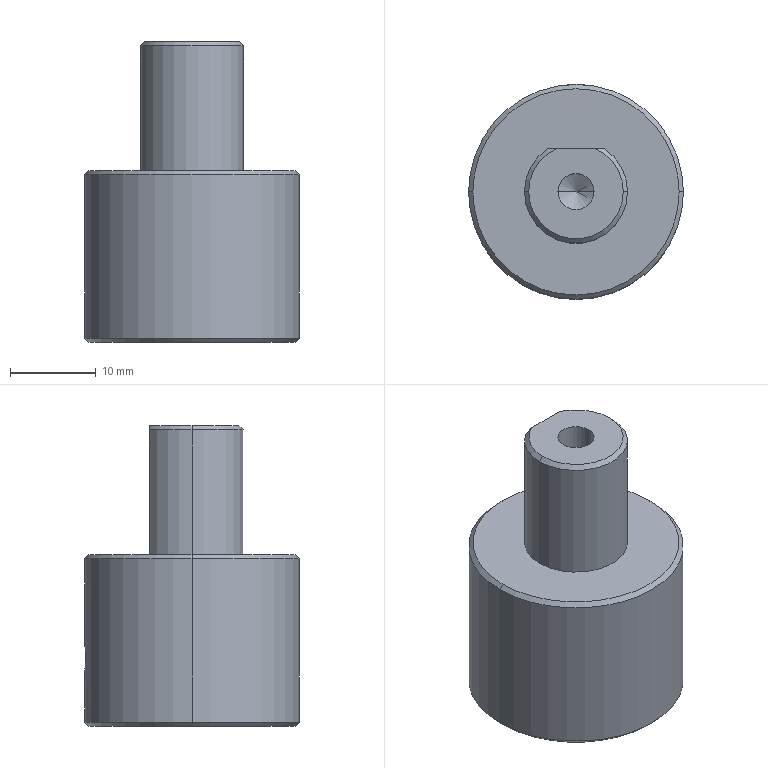Part | SolidWorks | features BaseBody 1 | 1 solid | 27 faces | box 25 x 25 x 35 mm | volume 8591 mm3 | cylinder 11 | cone 9 | plane 5 | torus 2 | commonest cylinder face diameters 12 x3 3.3 x2 4.2 x2 14 x2 25 x2
STEP:
#1=CARTESIAN_POINT('',(-2.1,0.,22.6));
#2=VERTEX_POINT('',#1);
#3=CARTESIAN_POINT('',(2.1,0.,22.6));
#4=VERTEX_POINT('',#3);
#5=CARTESIAN_POINT('',(0.,0.,22.6));
#6=DIRECTION('',(0.,0.,1.));
#7=DIRECTION('',(1.,0.,0.));
#8=AXIS2_PLACEMENT_3D('',#5,#6,#7);
#9=CIRCLE('',#8,2.1);
#10=EDGE_CURVE('',#2,#4,#9,.T.);
#11=ORIENTED_EDGE('',*,*,#10,.F.);
#12=CARTESIAN_POINT('',(-2.1,0.,35.));
#13=VERTEX_POINT('',#12);
#14=CARTESIAN_POINT('',(-2.1,0.,35.));
#15=DIRECTION('',(0.,0.,1.));
#16=VECTOR('',#15,1000.);
#17=LINE('',#14,#16);
#18=EDGE_CURVE('',#2,#13,#17,.T.);
#19=ORIENTED_EDGE('',*,*,#18,.T.);
#20=CARTESIAN_POINT('',(2.1,0.,35.));
#21=VERTEX_POINT('',#20);
#22=CARTESIAN_POINT('',(0.,0.,35.));
#23=DIRECTION('',(0.,0.,1.));
#24=DIRECTION('',(1.,0.,0.));
#25=AXIS2_PLACEMENT_3D('',#22,#23,#24);
#26=CIRCLE('',#25,2.1);
#27=EDGE_CURVE('',#13,#21,#26,.T.);
#28=ORIENTED_EDGE('',*,*,#27,.T.);
#29=CARTESIAN_POINT('',(2.1,0.,35.));
#30=DIRECTION('',(0.,0.,1.));
#31=VECTOR('',#30,1000.);
#32=LINE('',#29,#31);
#33=EDGE_CURVE('',#4,#21,#32,.T.);
#34=ORIENTED_EDGE('',*,*,#33,.F.);
#35=EDGE_LOOP('',(#11,#19,#28,#34));
#36=FACE_OUTER_BOUND('',#35,.T.);
#37=CARTESIAN_POINT('',(0.,0.,35.));
#38=DIRECTION('',(0.,0.,1.));
#39=DIRECTION('',(1.,0.,0.));
#40=AXIS2_PLACEMENT_3D('',#37,#38,#39);
#41=CYLINDRICAL_SURFACE('',#40,2.1);
#42=ADVANCED_FACE('',(#36),#41,.F.);
#43=CARTESIAN_POINT('',(0.,0.,21.338));
#44=VERTEX_POINT('',#43);
#45=CARTESIAN_POINT('',(2.1,0.,22.6));
#46=DIRECTION('',(0.8572,0.,0.515));
#47=VECTOR('',#46,1000.);
#48=LINE('',#45,#47);
#49=EDGE_CURVE('',#44,#4,#48,.T.);
#50=ORIENTED_EDGE('',*,*,#49,.F.);
#51=CARTESIAN_POINT('',(-2.1,0.,22.6));
#52=DIRECTION('',(-0.8572,0.,0.515));
#53=VECTOR('',#52,1000.);
#54=LINE('',#51,#53);
#55=EDGE_CURVE('',#44,#2,#54,.T.);
#56=ORIENTED_EDGE('',*,*,#55,.T.);
#57=ORIENTED_EDGE('',*,*,#10,.T.);
#58=EDGE_LOOP('',(#50,#56,#57));
#59=FACE_OUTER_BOUND('',#58,.T.);
#60=CARTESIAN_POINT('',(0.,0.,22.6));
#61=DIRECTION('',(0.,0.,1.));
#62=DIRECTION('',(1.,0.,0.));
#63=AXIS2_PLACEMENT_3D('',#60,#61,#62);
#64=CONICAL_SURFACE('',#63,2.1,1.03);
#65=ADVANCED_FACE('',(#59),#64,.F.);
#66=CARTESIAN_POINT('',(0.,12.5,9.65));
#67=VERTEX_POINT('',#66);
#68=CARTESIAN_POINT('',(0.,12.5,6.35));
#69=VERTEX_POINT('',#68);
#70=CARTESIAN_POINT('',(0.,12.5,9.65));
#71=CARTESIAN_POINT('',(-0.1091,12.5,9.65));
#72=CARTESIAN_POINT('',(-0.2164,12.499,9.639));
#73=CARTESIAN_POINT('',(-0.4274,12.493,9.597));
#74=CARTESIAN_POINT('',(-0.5323,12.489,9.566));
#75=CARTESIAN_POINT('',(-0.732,12.479,9.483));
#76=CARTESIAN_POINT('',(-0.8267,12.473,9.432));
#77=CARTESIAN_POINT('',(-1.006,12.46,9.312));
#78=CARTESIAN_POINT('',(-1.091,12.453,9.243));
#79=CARTESIAN_POINT('',(-1.319,12.431,9.015));
#80=CARTESIAN_POINT('',(-1.442,12.417,8.831));
#81=CARTESIAN_POINT('',(-1.606,12.397,8.434));
#82=CARTESIAN_POINT('',(-1.65,12.391,8.217));
#83=CARTESIAN_POINT('',(-1.65,12.391,7.893));
#84=CARTESIAN_POINT('',(-1.639,12.392,7.784));
#85=CARTESIAN_POINT('',(-1.597,12.398,7.572));
#86=CARTESIAN_POINT('',(-1.566,12.402,7.469));
#87=CARTESIAN_POINT('',(-1.483,12.412,7.27));
#88=CARTESIAN_POINT('',(-1.432,12.418,7.173));
#89=CARTESIAN_POINT('',(-1.313,12.431,6.994));
#90=CARTESIAN_POINT('',(-1.244,12.438,6.911));
#91=CARTESIAN_POINT('',(-1.091,12.453,6.757));
#92=CARTESIAN_POINT('',(-1.007,12.46,6.689));
#93=CARTESIAN_POINT('',(-0.8289,12.473,6.569));
#94=CARTESIAN_POINT('',(-0.7325,12.479,6.518));
#95=CARTESIAN_POINT('',(-0.4329,12.494,6.393));
#96=CARTESIAN_POINT('',(-0.2182,12.5,6.35));
#97=CARTESIAN_POINT('',(0.,12.5,6.35));
#98=B_SPLINE_CURVE_WITH_KNOTS('',3,(#70,#71,#72,#73,#74,#75,#76,#77,#78,#79,#80,#81,#82,#83,#84,#85,#86,#87,#88,#89,#90,#91,#92,#93,#94,#95,#96,#97),.UNSPECIFIED.,.F.,.F.,(4,2,2,2,2,2,2,2,2,2,2,2,2,4),(0.,0.0003227,0.0006454,0.0009681,0.001291,0.001936,0.002582,0.002904,0.003227,0.00355,0.003872,0.004195,0.004518,0.005163),.UNSPECIFIED.);
#99=EDGE_CURVE('',#67,#69,#98,.T.);
#100=ORIENTED_EDGE('',*,*,#99,.F.);
#101=CARTESIAN_POINT('',(0.,7.,9.65));
#102=VERTEX_POINT('',#101);
#103=CARTESIAN_POINT('',(0.,0.,9.65));
#104=DIRECTION('',(0.,-1.,0.));
#105=VECTOR('',#104,1000.);
#106=LINE('',#103,#105);
#107=EDGE_CURVE('',#67,#102,#106,.T.);
#108=ORIENTED_EDGE('',*,*,#107,.T.);
#109=CARTESIAN_POINT('',(0.,7.,6.35));
#110=VERTEX_POINT('',#109);
#111=CARTESIAN_POINT('',(0.,7.,6.35));
#112=CARTESIAN_POINT('',(-0.1094,7.,6.35));
#113=CARTESIAN_POINT('',(-0.2169,6.997,6.361));
#114=CARTESIAN_POINT('',(-0.4283,6.988,6.403));
#115=CARTESIAN_POINT('',(-0.5333,6.98,6.435));
#116=CARTESIAN_POINT('',(-0.7329,6.962,6.518));
#117=CARTESIAN_POINT('',(-0.8275,6.952,6.568));
#118=CARTESIAN_POINT('',(-1.007,6.928,6.688));
#119=CARTESIAN_POINT('',(-1.091,6.915,6.758));
#120=CARTESIAN_POINT('',(-1.318,6.876,6.985));
#121=CARTESIAN_POINT('',(-1.441,6.851,7.168));
#122=CARTESIAN_POINT('',(-1.606,6.814,7.565));
#123=CARTESIAN_POINT('',(-1.65,6.803,7.783));
#124=CARTESIAN_POINT('',(-1.65,6.803,8.107));
#125=CARTESIAN_POINT('',(-1.639,6.805,8.216));
#126=CARTESIAN_POINT('',(-1.597,6.815,8.428));
#127=CARTESIAN_POINT('',(-1.566,6.823,8.531));
#128=CARTESIAN_POINT('',(-1.441,6.85,8.832));
#129=CARTESIAN_POINT('',(-1.32,6.876,9.013));
#130=CARTESIAN_POINT('',(-1.091,6.915,9.243));
#131=CARTESIAN_POINT('',(-1.008,6.928,9.311));
#132=CARTESIAN_POINT('',(-0.8298,6.951,9.43));
#133=CARTESIAN_POINT('',(-0.7332,6.962,9.482));
#134=CARTESIAN_POINT('',(-0.4344,6.989,9.606));
#135=CARTESIAN_POINT('',(-0.2188,7.,9.65));
#136=CARTESIAN_POINT('',(0.,7.,9.65));
#137=B_SPLINE_CURVE_WITH_KNOTS('',3,(#111,#112,#113,#114,#115,#116,#117,#118,#119,#120,#121,#122,#123,#124,#125,#126,#127,#128,#129,#130,#131,#132,#133,#134,#135,#136),.UNSPECIFIED.,.F.,.F.,(4,2,2,2,2,2,2,2,2,2,2,2,4),(0.,0.0003235,0.0006469,0.0009704,0.001294,0.001941,0.002588,0.002911,0.003235,0.003882,0.004205,0.004528,0.005175),.UNSPECIFIED.);
#138=EDGE_CURVE('',#110,#102,#137,.T.);
#139=ORIENTED_EDGE('',*,*,#138,.F.);
#140=CARTESIAN_POINT('',(0.,0.,6.35));
#141=DIRECTION('',(0.,-1.,0.));
#142=VECTOR('',#141,1000.);
#143=LINE('',#140,#142);
#144=EDGE_CURVE('',#69,#110,#143,.T.);
#145=ORIENTED_EDGE('',*,*,#144,.F.);
#146=EDGE_LOOP('',(#100,#108,#139,#145));
#147=FACE_OUTER_BOUND('',#146,.T.);
#148=CARTESIAN_POINT('',(0.,0.,8.));
#149=DIRECTION('',(0.,-1.,0.));
#150=DIRECTION('',(0.,0.,-1.));
#151=AXIS2_PLACEMENT_3D('',#148,#149,#150);
#152=CYLINDRICAL_SURFACE('',#151,1.65);
#153=ADVANCED_FACE('',(#147),#152,.F.);
#154=CARTESIAN_POINT('',(-12.,0.,0.));
#155=VERTEX_POINT('',#154);
#156=CARTESIAN_POINT('',(12.,0.,0.));
#157=VERTEX_POINT('',#156);
#158=CARTESIAN_POINT('',(0.,0.,0.));
#159=DIRECTION('',(0.,0.,-1.));
#160=DIRECTION('',(1.,0.,0.));
#161=AXIS2_PLACEMENT_3D('',#158,#159,#160);
#162=CIRCLE('',#161,12.);
#163=EDGE_CURVE('',#155,#157,#162,.T.);
#164=ORIENTED_EDGE('',*,*,#163,.F.);
#165=CARTESIAN_POINT('',(-12.5,0.,0.5));
#166=VERTEX_POINT('',#165);
#167=CARTESIAN_POINT('',(-12.5,0.,0.5));
#168=DIRECTION('',(-0.7071,0.,0.7071));
#169=VECTOR('',#168,1000.);
#170=LINE('',#167,#169);
#171=EDGE_CURVE('',#155,#166,#170,.T.);
#172=ORIENTED_EDGE('',*,*,#171,.T.);
#173=CARTESIAN_POINT('',(12.5,0.,0.5));
#174=VERTEX_POINT('',#173);
#175=CARTESIAN_POINT('',(0.,0.,0.5));
#176=DIRECTION('',(0.,0.,1.));
#177=DIRECTION('',(1.,0.,0.));
#178=AXIS2_PLACEMENT_3D('',#175,#176,#177);
#179=CIRCLE('',#178,12.5);
#180=EDGE_CURVE('',#174,#166,#179,.T.);
#181=ORIENTED_EDGE('',*,*,#180,.F.);
#182=CARTESIAN_POINT('',(12.5,0.,0.5));
#183=DIRECTION('',(0.7071,0.,0.7071));
#184=VECTOR('',#183,1000.);
#185=LINE('',#182,#184);
#186=EDGE_CURVE('',#157,#174,#185,.T.);
#187=ORIENTED_EDGE('',*,*,#186,.F.);
#188=EDGE_LOOP('',(#164,#172,#181,#187));
#189=FACE_OUTER_BOUND('',#188,.T.);
#190=CARTESIAN_POINT('',(0.,0.,0.5));
#191=DIRECTION('',(0.,0.,1.));
#192=DIRECTION('',(1.,0.,0.));
#193=AXIS2_PLACEMENT_3D('',#190,#191,#192);
#194=CONICAL_SURFACE('',#193,12.5,0.7854);
#195=ADVANCED_FACE('',(#189),#194,.T.);
#196=CARTESIAN_POINT('',(12.,0.,20.));
#197=VERTEX_POINT('',#196);
#198=CARTESIAN_POINT('',(-12.,0.,20.));
#199=VERTEX_POINT('',#198);
#200=CARTESIAN_POINT('',(0.,0.,20.));
#201=DIRECTION('',(0.,0.,1.));
#202=DIRECTION('',(1.,0.,0.));
#203=AXIS2_PLACEMENT_3D('',#200,#201,#202);
#204=CIRCLE('',#203,12.);
#205=EDGE_CURVE('',#197,#199,#204,.T.);
#206=ORIENTED_EDGE('',*,*,#205,.F.);
#207=CARTESIAN_POINT('',(12.5,0.,19.5));
#208=VERTEX_POINT('',#207);
#209=CARTESIAN_POINT('',(12.,0.,20.));
#210=DIRECTION('',(0.7071,0.,-0.7071));
#211=VECTOR('',#210,1000.);
#212=LINE('',#209,#211);
#213=EDGE_CURVE('',#197,#208,#212,.T.);
#214=ORIENTED_EDGE('',*,*,#213,.T.);
#215=CARTESIAN_POINT('',(-12.5,0.,19.5));
#216=VERTEX_POINT('',#215);
#217=CARTESIAN_POINT('',(0.,0.,19.5));
#218=DIRECTION('',(0.,0.,-1.));
#219=DIRECTION('',(1.,0.,0.));
#220=AXIS2_PLACEMENT_3D('',#217,#218,#219);
#221=CIRCLE('',#220,12.5);
#222=EDGE_CURVE('',#216,#208,#221,.T.);
#223=ORIENTED_EDGE('',*,*,#222,.F.);
#224=CARTESIAN_POINT('',(-12.,0.,20.));
#225=DIRECTION('',(-0.7071,0.,-0.7071));
#226=VECTOR('',#225,1000.);
#227=LINE('',#224,#226);
#228=EDGE_CURVE('',#199,#216,#227,.T.);
#229=ORIENTED_EDGE('',*,*,#228,.F.);
#230=EDGE_LOOP('',(#206,#214,#223,#229));
#231=FACE_OUTER_BOUND('',#230,.T.);
#232=CARTESIAN_POINT('',(0.,0.,20.));
#233=DIRECTION('',(0.,0.,-1.));
#234=DIRECTION('',(-1.,0.,0.));
#235=AXIS2_PLACEMENT_3D('',#232,#233,#234);
#236=CONICAL_SURFACE('',#235,12.,0.7854);
#237=ADVANCED_FACE('',(#231),#236,.T.);
#238=CARTESIAN_POINT('',(5.5,0.,35.));
#239=VERTEX_POINT('',#238);
#240=CARTESIAN_POINT('',(2.291,5.,35.));
#241=VERTEX_POINT('',#240);
#242=CARTESIAN_POINT('',(0.,0.,35.));
#243=DIRECTION('',(0.,0.,1.));
#244=DIRECTION('',(-1.,0.,0.));
#245=AXIS2_PLACEMENT_3D('',#242,#243,#244);
#246=CIRCLE('',#245,5.5);
#247=EDGE_CURVE('',#239,#241,#246,.T.);
#248=ORIENTED_EDGE('',*,*,#247,.F.);
#249=CARTESIAN_POINT('',(6.,0.,34.5));
#250=VERTEX_POINT('',#249);
#251=CARTESIAN_POINT('',(5.5,0.,35.));
#252=DIRECTION('',(0.7071,0.,-0.7071));
#253=VECTOR('',#252,1000.);
#254=LINE('',#251,#253);
#255=EDGE_CURVE('',#239,#250,#254,.T.);
#256=ORIENTED_EDGE('',*,*,#255,.T.);
#257=CARTESIAN_POINT('',(3.317,5.,34.5));
#258=VERTEX_POINT('',#257);
#259=CARTESIAN_POINT('',(0.,0.,34.5));
#260=DIRECTION('',(0.,0.,-1.));
#261=DIRECTION('',(-1.,0.,0.));
#262=AXIS2_PLACEMENT_3D('',#259,#260,#261);
#263=CIRCLE('',#262,6.);
#264=EDGE_CURVE('',#258,#250,#263,.T.);
#265=ORIENTED_EDGE('',*,*,#264,.F.);
#266=CARTESIAN_POINT('',(2.291,5.,35.));
#267=CARTESIAN_POINT('',(2.643,5.,34.854));
#268=CARTESIAN_POINT('',(2.983,5.,34.684));
#269=CARTESIAN_POINT('',(3.317,5.,34.5));
#270=B_SPLINE_CURVE_WITH_KNOTS('',3,(#266,#267,#268,#269),.UNSPECIFIED.,.F.,.F.,(4,4),(0.,0.001141),.UNSPECIFIED.);
#271=EDGE_CURVE('',#241,#258,#270,.T.);
#272=ORIENTED_EDGE('',*,*,#271,.F.);
#273=EDGE_LOOP('',(#248,#256,#265,#272));
#274=FACE_OUTER_BOUND('',#273,.T.);
#275=CARTESIAN_POINT('',(0.,0.,35.));
#276=DIRECTION('',(0.,0.,-1.));
#277=DIRECTION('',(-1.,0.,0.));
#278=AXIS2_PLACEMENT_3D('',#275,#276,#277);
#279=CONICAL_SURFACE('',#278,5.5,0.7854);
#280=ADVANCED_FACE('',(#274),#279,.T.);
#281=ORIENTED_EDGE('',*,*,#255,.F.);
#282=CARTESIAN_POINT('',(-5.5,0.,35.));
#283=VERTEX_POINT('',#282);
#284=CARTESIAN_POINT('',(0.,0.,35.));
#285=DIRECTION('',(0.,0.,1.));
#286=DIRECTION('',(-1.,0.,0.));
#287=AXIS2_PLACEMENT_3D('',#284,#285,#286);
#288=CIRCLE('',#287,5.5);
#289=EDGE_CURVE('',#283,#239,#288,.T.);
#290=ORIENTED_EDGE('',*,*,#289,.F.);
#291=CARTESIAN_POINT('',(-6.,0.,34.5));
#292=VERTEX_POINT('',#291);
#293=CARTESIAN_POINT('',(-5.5,0.,35.));
#294=DIRECTION('',(-0.7071,0.,-0.7071));
#295=VECTOR('',#294,1000.);
#296=LINE('',#293,#295);
#297=EDGE_CURVE('',#283,#292,#296,.T.);
#298=ORIENTED_EDGE('',*,*,#297,.T.);
#299=CARTESIAN_POINT('',(0.,0.,34.5));
#300=DIRECTION('',(0.,0.,-1.));
#301=DIRECTION('',(-1.,0.,0.));
#302=AXIS2_PLACEMENT_3D('',#299,#300,#301);
#303=CIRCLE('',#302,6.);
#304=EDGE_CURVE('',#250,#292,#303,.T.);
#305=ORIENTED_EDGE('',*,*,#304,.F.);
#306=EDGE_LOOP('',(#281,#290,#298,#305));
#307=FACE_OUTER_BOUND('',#306,.T.);
#308=CARTESIAN_POINT('',(0.,0.,35.));
#309=DIRECTION('',(0.,0.,-1.));
#310=DIRECTION('',(-1.,0.,0.));
#311=AXIS2_PLACEMENT_3D('',#308,#309,#310);
#312=CONICAL_SURFACE('',#311,5.5,0.7854);
#313=ADVANCED_FACE('',(#307),#312,.T.);
#314=CARTESIAN_POINT('',(6.,0.,17.));
#315=VERTEX_POINT('',#314);
#316=CARTESIAN_POINT('',(-6.,0.,17.));
#317=VERTEX_POINT('',#316);
#318=CARTESIAN_POINT('',(0.,0.,17.));
#319=DIRECTION('',(0.,0.,-1.));
#320=DIRECTION('',(-1.,0.,0.));
#321=AXIS2_PLACEMENT_3D('',#318,#319,#320);
#322=CIRCLE('',#321,6.);
#323=EDGE_CURVE('',#315,#317,#322,.T.);
#324=ORIENTED_EDGE('',*,*,#323,.F.);
#325=CARTESIAN_POINT('',(7.,0.,16.));
#326=VERTEX_POINT('',#325);
#327=CARTESIAN_POINT('',(6.,0.,16.));
#328=DIRECTION('',(0.,1.,0.));
#329=DIRECTION('',(-1.,0.,0.));
#330=AXIS2_PLACEMENT_3D('',#327,#328,#329);
#331=CIRCLE('',#330,1.);
#332=EDGE_CURVE('',#315,#326,#331,.T.);
#333=ORIENTED_EDGE('',*,*,#332,.T.);
#334=CARTESIAN_POINT('',(-7.,0.,16.));
#335=VERTEX_POINT('',#334);
#336=CARTESIAN_POINT('',(0.,0.,16.));
#337=DIRECTION('',(0.,0.,1.));
#338=DIRECTION('',(-1.,0.,0.));
#339=AXIS2_PLACEMENT_3D('',#336,#337,#338);
#340=CIRCLE('',#339,7.);
#341=EDGE_CURVE('',#335,#326,#340,.T.);
#342=ORIENTED_EDGE('',*,*,#341,.F.);
#343=CARTESIAN_POINT('',(-6.,0.,16.));
#344=DIRECTION('',(0.,-1.,0.));
#345=DIRECTION('',(0.,0.,-1.));
#346=AXIS2_PLACEMENT_3D('',#343,#344,#345);
#347=CIRCLE('',#346,1.);
#348=EDGE_CURVE('',#317,#335,#347,.T.);
#349=ORIENTED_EDGE('',*,*,#348,.F.);
#350=EDGE_LOOP('',(#324,#333,#342,#349));
#351=FACE_OUTER_BOUND('',#350,.T.);
#352=CARTESIAN_POINT('',(0.,0.,16.));
#353=DIRECTION('',(0.,0.,-1.));
#354=DIRECTION('',(-1.,0.,0.));
#355=AXIS2_PLACEMENT_3D('',#352,#353,#354);
#356=TOROIDAL_SURFACE('',#355,6.,1.);
#357=ADVANCED_FACE('',(#351),#356,.F.);
#358=ORIENTED_EDGE('',*,*,#341,.T.);
#359=CARTESIAN_POINT('',(7.,0.,0.));
#360=VERTEX_POINT('',#359);
#361=CARTESIAN_POINT('',(7.,0.,17.));
#362=DIRECTION('',(0.,0.,-1.));
#363=VECTOR('',#362,1000.);
#364=LINE('',#361,#363);
#365=EDGE_CURVE('',#326,#360,#364,.T.);
#366=ORIENTED_EDGE('',*,*,#365,.T.);
#367=CARTESIAN_POINT('',(-7.,0.,0.));
#368=VERTEX_POINT('',#367);
#369=CARTESIAN_POINT('',(0.,0.,0.));
#370=DIRECTION('',(0.,0.,-1.));
#371=DIRECTION('',(-1.,0.,0.));
#372=AXIS2_PLACEMENT_3D('',#369,#370,#371);
#373=CIRCLE('',#372,7.);
#374=EDGE_CURVE('',#360,#368,#373,.T.);
#375=ORIENTED_EDGE('',*,*,#374,.T.);
#376=CARTESIAN_POINT('',(-7.,0.,17.));
#377=DIRECTION('',(0.,0.,-1.));
#378=VECTOR('',#377,1000.);
#379=LINE('',#376,#378);
#380=EDGE_CURVE('',#335,#368,#379,.T.);
#381=ORIENTED_EDGE('',*,*,#380,.F.);
#382=EDGE_LOOP('',(#358,#366,#375,#381));
#383=FACE_OUTER_BOUND('',#382,.T.);
#384=CARTESIAN_POINT('',(0.,0.,17.));
#385=DIRECTION('',(0.,0.,-1.));
#386=DIRECTION('',(-1.,0.,0.));
#387=AXIS2_PLACEMENT_3D('',#384,#385,#386);
#388=CYLINDRICAL_SURFACE('',#387,7.);
#389=ADVANCED_FACE('',(#383),#388,.F.);
#390=ORIENTED_EDGE('',*,*,#264,.T.);
#391=CARTESIAN_POINT('',(6.,0.,20.));
#392=VERTEX_POINT('',#391);
#393=CARTESIAN_POINT('',(6.,0.,35.));
#394=DIRECTION('',(0.,0.,-1.));
#395=VECTOR('',#394,1000.);
#396=LINE('',#393,#395);
#397=EDGE_CURVE('',#250,#392,#396,.T.);
#398=ORIENTED_EDGE('',*,*,#397,.T.);
#399=CARTESIAN_POINT('',(3.317,5.,20.));
#400=VERTEX_POINT('',#399);
#401=CARTESIAN_POINT('',(0.,0.,20.));
#402=DIRECTION('',(0.,0.,1.));
#403=DIRECTION('',(-1.,0.,0.));
#404=AXIS2_PLACEMENT_3D('',#401,#402,#403);
#405=CIRCLE('',#404,6.);
#406=EDGE_CURVE('',#392,#400,#405,.T.);
#407=ORIENTED_EDGE('',*,*,#406,.T.);
#408=CARTESIAN_POINT('',(3.317,5.,35.));
#409=DIRECTION('',(0.,0.,-1.));
#410=VECTOR('',#409,1000.);
#411=LINE('',#408,#410);
#412=EDGE_CURVE('',#258,#400,#411,.T.);
#413=ORIENTED_EDGE('',*,*,#412,.F.);
#414=EDGE_LOOP('',(#390,#398,#407,#413));
#415=FACE_OUTER_BOUND('',#414,.T.);
#416=CARTESIAN_POINT('',(0.,0.,35.));
#417=DIRECTION('',(0.,0.,-1.));
#418=DIRECTION('',(-1.,0.,0.));
#419=AXIS2_PLACEMENT_3D('',#416,#417,#418);
#420=CYLINDRICAL_SURFACE('',#419,6.);
#421=ADVANCED_FACE('',(#415),#420,.T.);
#422=ORIENTED_EDGE('',*,*,#397,.F.);
#423=ORIENTED_EDGE('',*,*,#304,.T.);
#424=CARTESIAN_POINT('',(-6.,0.,20.));
#425=VERTEX_POINT('',#424);
#426=CARTESIAN_POINT('',(-6.,0.,35.));
#427=DIRECTION('',(0.,0.,-1.));
#428=VECTOR('',#427,1000.);
#429=LINE('',#426,#428);
#430=EDGE_CURVE('',#292,#425,#429,.T.);
#431=ORIENTED_EDGE('',*,*,#430,.T.);
#432=CARTESIAN_POINT('',(0.,0.,20.));
#433=DIRECTION('',(0.,0.,1.));
#434=DIRECTION('',(-1.,0.,0.));
#435=AXIS2_PLACEMENT_3D('',#432,#433,#434);
#436=CIRCLE('',#435,6.);
#437=EDGE_CURVE('',#425,#392,#436,.T.);
#438=ORIENTED_EDGE('',*,*,#437,.T.);
#439=EDGE_LOOP('',(#422,#423,#431,#438));
#440=FACE_OUTER_BOUND('',#439,.T.);
#441=CARTESIAN_POINT('',(0.,0.,35.));
#442=DIRECTION('',(0.,0.,-1.));
#443=DIRECTION('',(-1.,0.,0.));
#444=AXIS2_PLACEMENT_3D('',#441,#442,#443);
#445=CYLINDRICAL_SURFACE('',#444,6.);
#446=ADVANCED_FACE('',(#440),#445,.T.);
#447=CARTESIAN_POINT('',(0.,12.5,6.35));
#448=CARTESIAN_POINT('',(0.1091,12.5,6.35));
#449=CARTESIAN_POINT('',(0.2164,12.499,6.361));
#450=CARTESIAN_POINT('',(0.4274,12.493,6.403));
#451=CARTESIAN_POINT('',(0.5323,12.489,6.434));
#452=CARTESIAN_POINT('',(0.732,12.479,6.517));
#453=CARTESIAN_POINT('',(0.8267,12.473,6.568));
#454=CARTESIAN_POINT('',(1.006,12.46,6.688));
#455=CARTESIAN_POINT('',(1.091,12.453,6.757));
#456=CARTESIAN_POINT('',(1.319,12.431,6.985));
#457=CARTESIAN_POINT('',(1.442,12.417,7.169));
#458=CARTESIAN_POINT('',(1.606,12.397,7.566));
#459=CARTESIAN_POINT('',(1.65,12.391,7.783));
#460=CARTESIAN_POINT('',(1.65,12.391,8.107));
#461=CARTESIAN_POINT('',(1.639,12.392,8.216));
#462=CARTESIAN_POINT('',(1.597,12.398,8.428));
#463=CARTESIAN_POINT('',(1.566,12.402,8.531));
#464=CARTESIAN_POINT('',(1.483,12.412,8.73));
#465=CARTESIAN_POINT('',(1.432,12.418,8.827));
#466=CARTESIAN_POINT('',(1.313,12.431,9.006));
#467=CARTESIAN_POINT('',(1.244,12.438,9.089));
#468=CARTESIAN_POINT('',(1.091,12.453,9.243));
#469=CARTESIAN_POINT('',(1.007,12.46,9.311));
#470=CARTESIAN_POINT('',(0.8289,12.473,9.431));
#471=CARTESIAN_POINT('',(0.7325,12.479,9.482));
#472=CARTESIAN_POINT('',(0.4329,12.494,9.607));
#473=CARTESIAN_POINT('',(0.2182,12.5,9.65));
#474=CARTESIAN_POINT('',(0.,12.5,9.65));
#475=B_SPLINE_CURVE_WITH_KNOTS('',3,(#447,#448,#449,#450,#451,#452,#453,#454,#455,#456,#457,#458,#459,#460,#461,#462,#463,#464,#465,#466,#467,#468,#469,#470,#471,#472,#473,#474),.UNSPECIFIED.,.F.,.F.,(4,2,2,2,2,2,2,2,2,2,2,2,2,4),(0.005163,0.005486,0.005808,0.006131,0.006454,0.007099,0.007745,0.008067,0.00839,0.008713,0.009035,0.009358,0.009681,0.01033),.UNSPECIFIED.);
#476=EDGE_CURVE('',#69,#67,#475,.T.);
#477=ORIENTED_EDGE('',*,*,#476,.T.);
#478=ORIENTED_EDGE('',*,*,#99,.T.);
#479=EDGE_LOOP('',(#477,#478));
#480=FACE_BOUND('',#479,.T.);
#481=ORIENTED_EDGE('',*,*,#222,.T.);
#482=CARTESIAN_POINT('',(12.5,0.,20.));
#483=DIRECTION('',(0.,0.,-1.));
#484=VECTOR('',#483,1000.);
#485=LINE('',#482,#484);
#486=EDGE_CURVE('',#208,#174,#485,.T.);
#487=ORIENTED_EDGE('',*,*,#486,.T.);
#488=ORIENTED_EDGE('',*,*,#180,.T.);
#489=CARTESIAN_POINT('',(-12.5,0.,20.));
#490=DIRECTION('',(0.,0.,-1.));
#491=VECTOR('',#490,1000.);
#492=LINE('',#489,#491);
#493=EDGE_CURVE('',#216,#166,#492,.T.);
#494=ORIENTED_EDGE('',*,*,#493,.F.);
#495=EDGE_LOOP('',(#481,#487,#488,#494));
#496=FACE_OUTER_BOUND('',#495,.T.);
#497=CARTESIAN_POINT('',(0.,0.,20.));
#498=DIRECTION('',(0.,0.,-1.));
#499=DIRECTION('',(-1.,0.,0.));
#500=AXIS2_PLACEMENT_3D('',#497,#498,#499);
#501=CYLINDRICAL_SURFACE('',#500,12.5);
#502=ADVANCED_FACE('',(#480,#496),#501,.T.);
#503=CARTESIAN_POINT('',(0.,0.,17.));
#504=DIRECTION('',(0.,0.,-1.));
#505=DIRECTION('',(-1.,0.,0.));
#506=AXIS2_PLACEMENT_3D('',#503,#504,#505);
#507=CIRCLE('',#506,6.);
#508=EDGE_CURVE('',#317,#315,#507,.T.);
#509=ORIENTED_EDGE('',*,*,#508,.T.);
#510=ORIENTED_EDGE('',*,*,#323,.T.);
#511=EDGE_LOOP('',(#509,#510));
#512=FACE_OUTER_BOUND('',#511,.T.);
#513=CARTESIAN_POINT('',(0.,0.,17.));
#514=DIRECTION('',(0.,0.,-1.));
#515=DIRECTION('',(0.,-1.,0.));
#516=AXIS2_PLACEMENT_3D('',#513,#514,#515);
#517=PLANE('',#516);
#518=ADVANCED_FACE('',(#512),#517,.T.);
#519=CARTESIAN_POINT('',(0.,0.,35.));
#520=DIRECTION('',(0.,0.,1.));
#521=DIRECTION('',(1.,0.,0.));
#522=AXIS2_PLACEMENT_3D('',#519,#520,#521);
#523=CIRCLE('',#522,2.1);
#524=EDGE_CURVE('',#21,#13,#523,.T.);
#525=ORIENTED_EDGE('',*,*,#524,.F.);
#526=ORIENTED_EDGE('',*,*,#27,.F.);
#527=EDGE_LOOP('',(#525,#526));
#528=FACE_BOUND('',#527,.T.);
#529=CARTESIAN_POINT('',(-2.291,5.,35.));
#530=VERTEX_POINT('',#529);
#531=CARTESIAN_POINT('',(3.317,5.,35.));
#532=DIRECTION('',(-1.,0.,0.));
#533=VECTOR('',#532,1000.);
#534=LINE('',#531,#533);
#535=EDGE_CURVE('',#241,#530,#534,.T.);
#536=ORIENTED_EDGE('',*,*,#535,.T.);
#537=CARTESIAN_POINT('',(0.,0.,35.));
#538=DIRECTION('',(0.,0.,1.));
#539=DIRECTION('',(-1.,0.,0.));
#540=AXIS2_PLACEMENT_3D('',#537,#538,#539);
#541=CIRCLE('',#540,5.5);
#542=EDGE_CURVE('',#530,#283,#541,.T.);
#543=ORIENTED_EDGE('',*,*,#542,.T.);
#544=ORIENTED_EDGE('',*,*,#289,.T.);
#545=ORIENTED_EDGE('',*,*,#247,.T.);
#546=EDGE_LOOP('',(#536,#543,#544,#545));
#547=FACE_OUTER_BOUND('',#546,.T.);
#548=CARTESIAN_POINT('',(0.,0.,35.));
#549=DIRECTION('',(0.,0.,-1.));
#550=DIRECTION('',(0.,-1.,0.));
#551=AXIS2_PLACEMENT_3D('',#548,#549,#550);
#552=PLANE('',#551);
#553=ADVANCED_FACE('',(#528,#547),#552,.F.);
#554=ORIENTED_EDGE('',*,*,#535,.F.);
#555=ORIENTED_EDGE('',*,*,#271,.T.);
#556=ORIENTED_EDGE('',*,*,#412,.T.);
#557=CARTESIAN_POINT('',(-3.317,5.,20.));
#558=VERTEX_POINT('',#557);
#559=CARTESIAN_POINT('',(3.317,5.,20.));
#560=DIRECTION('',(-1.,0.,0.));
#561=VECTOR('',#560,1000.);
#562=LINE('',#559,#561);
#563=EDGE_CURVE('',#400,#558,#562,.T.);
#564=ORIENTED_EDGE('',*,*,#563,.T.);
#565=CARTESIAN_POINT('',(-3.317,5.,34.5));
#566=VERTEX_POINT('',#565);
#567=CARTESIAN_POINT('',(-3.317,5.,35.));
#568=DIRECTION('',(0.,0.,-1.));
#569=VECTOR('',#568,1000.);
#570=LINE('',#567,#569);
#571=EDGE_CURVE('',#566,#558,#570,.T.);
#572=ORIENTED_EDGE('',*,*,#571,.F.);
#573=CARTESIAN_POINT('',(-3.317,5.,34.5));
#574=CARTESIAN_POINT('',(-2.983,5.,34.684));
#575=CARTESIAN_POINT('',(-2.643,5.,34.854));
#576=CARTESIAN_POINT('',(-2.291,5.,35.));
#577=B_SPLINE_CURVE_WITH_KNOTS('',3,(#573,#574,#575,#576),.UNSPECIFIED.,.F.,.F.,(4,4),(0.,0.001141),.UNSPECIFIED.);
#578=EDGE_CURVE('',#566,#530,#577,.T.);
#579=ORIENTED_EDGE('',*,*,#578,.T.);
#580=EDGE_LOOP('',(#554,#555,#556,#564,#572,#579));
#581=FACE_OUTER_BOUND('',#580,.T.);
#582=CARTESIAN_POINT('',(3.317,5.,35.));
#583=DIRECTION('',(0.,-1.,0.));
#584=DIRECTION('',(0.,0.,-1.));
#585=AXIS2_PLACEMENT_3D('',#582,#583,#584);
#586=PLANE('',#585);
#587=ADVANCED_FACE('',(#581),#586,.F.);
#588=CARTESIAN_POINT('',(0.,0.,0.));
#589=DIRECTION('',(0.,0.,-1.));
#590=DIRECTION('',(-1.,0.,0.));
#591=AXIS2_PLACEMENT_3D('',#588,#589,#590);
#592=CIRCLE('',#591,7.);
#593=EDGE_CURVE('',#368,#360,#592,.T.);
#594=ORIENTED_EDGE('',*,*,#593,.F.);
#595=ORIENTED_EDGE('',*,*,#374,.F.);
#596=EDGE_LOOP('',(#594,#595));
#597=FACE_BOUND('',#596,.T.);
#598=CARTESIAN_POINT('',(0.,0.,0.));
#599=DIRECTION('',(0.,0.,-1.));
#600=DIRECTION('',(1.,0.,0.));
#601=AXIS2_PLACEMENT_3D('',#598,#599,#600);
#602=CIRCLE('',#601,12.);
#603=EDGE_CURVE('',#157,#155,#602,.T.);
#604=ORIENTED_EDGE('',*,*,#603,.T.);
#605=ORIENTED_EDGE('',*,*,#163,.T.);
#606=EDGE_LOOP('',(#604,#605));
#607=FACE_OUTER_BOUND('',#606,.T.);
#608=CARTESIAN_POINT('',(0.,0.,0.));
#609=DIRECTION('',(0.,0.,1.));
#610=DIRECTION('',(1.,0.,0.));
#611=AXIS2_PLACEMENT_3D('',#608,#609,#610);
#612=PLANE('',#611);
#613=ADVANCED_FACE('',(#597,#607),#612,.F.);
#614=CARTESIAN_POINT('',(0.,0.,20.));
#615=DIRECTION('',(0.,0.,1.));
#616=DIRECTION('',(-1.,0.,0.));
#617=AXIS2_PLACEMENT_3D('',#614,#615,#616);
#618=CIRCLE('',#617,6.);
#619=EDGE_CURVE('',#558,#425,#618,.T.);
#620=ORIENTED_EDGE('',*,*,#619,.F.);
#621=ORIENTED_EDGE('',*,*,#563,.F.);
#622=ORIENTED_EDGE('',*,*,#406,.F.);
#623=ORIENTED_EDGE('',*,*,#437,.F.);
#624=EDGE_LOOP('',(#620,#621,#622,#623));
#625=FACE_BOUND('',#624,.T.);
#626=CARTESIAN_POINT('',(0.,0.,20.));
#627=DIRECTION('',(0.,0.,1.));
#628=DIRECTION('',(1.,0.,0.));
#629=AXIS2_PLACEMENT_3D('',#626,#627,#628);
#630=CIRCLE('',#629,12.);
#631=EDGE_CURVE('',#199,#197,#630,.T.);
#632=ORIENTED_EDGE('',*,*,#631,.T.);
#633=ORIENTED_EDGE('',*,*,#205,.T.);
#634=EDGE_LOOP('',(#632,#633));
#635=FACE_OUTER_BOUND('',#634,.T.);
#636=CARTESIAN_POINT('',(0.,0.,20.));
#637=DIRECTION('',(0.,0.,1.));
#638=DIRECTION('',(1.,0.,0.));
#639=AXIS2_PLACEMENT_3D('',#636,#637,#638);
#640=PLANE('',#639);
#641=ADVANCED_FACE('',(#625,#635),#640,.T.);
#642=ORIENTED_EDGE('',*,*,#486,.F.);
#643=CARTESIAN_POINT('',(0.,0.,19.5));
#644=DIRECTION('',(0.,0.,-1.));
#645=DIRECTION('',(1.,0.,0.));
#646=AXIS2_PLACEMENT_3D('',#643,#644,#645);
#647=CIRCLE('',#646,12.5);
#648=EDGE_CURVE('',#208,#216,#647,.T.);
#649=ORIENTED_EDGE('',*,*,#648,.T.);
#650=ORIENTED_EDGE('',*,*,#493,.T.);
#651=CARTESIAN_POINT('',(0.,0.,0.5));
#652=DIRECTION('',(0.,0.,1.));
#653=DIRECTION('',(1.,0.,0.));
#654=AXIS2_PLACEMENT_3D('',#651,#652,#653);
#655=CIRCLE('',#654,12.5);
#656=EDGE_CURVE('',#166,#174,#655,.T.);
#657=ORIENTED_EDGE('',*,*,#656,.T.);
#658=EDGE_LOOP('',(#642,#649,#650,#657));
#659=FACE_OUTER_BOUND('',#658,.T.);
#660=CARTESIAN_POINT('',(0.,0.,20.));
#661=DIRECTION('',(0.,0.,-1.));
#662=DIRECTION('',(-1.,0.,0.));
#663=AXIS2_PLACEMENT_3D('',#660,#661,#662);
#664=CYLINDRICAL_SURFACE('',#663,12.5);
#665=ADVANCED_FACE('',(#659),#664,.T.);
#666=ORIENTED_EDGE('',*,*,#430,.F.);
#667=CARTESIAN_POINT('',(0.,0.,34.5));
#668=DIRECTION('',(0.,0.,-1.));
#669=DIRECTION('',(-1.,0.,0.));
#670=AXIS2_PLACEMENT_3D('',#667,#668,#669);
#671=CIRCLE('',#670,6.);
#672=EDGE_CURVE('',#292,#566,#671,.T.);
#673=ORIENTED_EDGE('',*,*,#672,.T.);
#674=ORIENTED_EDGE('',*,*,#571,.T.);
#675=ORIENTED_EDGE('',*,*,#619,.T.);
#676=EDGE_LOOP('',(#666,#673,#674,#675));
#677=FACE_OUTER_BOUND('',#676,.T.);
#678=CARTESIAN_POINT('',(0.,0.,35.));
#679=DIRECTION('',(0.,0.,-1.));
#680=DIRECTION('',(-1.,0.,0.));
#681=AXIS2_PLACEMENT_3D('',#678,#679,#680);
#682=CYLINDRICAL_SURFACE('',#681,6.);
#683=ADVANCED_FACE('',(#677),#682,.T.);
#684=ORIENTED_EDGE('',*,*,#365,.F.);
#685=CARTESIAN_POINT('',(0.,0.,16.));
#686=DIRECTION('',(0.,0.,1.));
#687=DIRECTION('',(-1.,0.,0.));
#688=AXIS2_PLACEMENT_3D('',#685,#686,#687);
#689=CIRCLE('',#688,7.);
#690=EDGE_CURVE('',#326,#335,#689,.T.);
#691=ORIENTED_EDGE('',*,*,#690,.T.);
#692=ORIENTED_EDGE('',*,*,#380,.T.);
#693=ORIENTED_EDGE('',*,*,#593,.T.);
#694=EDGE_LOOP('',(#684,#691,#692,#693));
#695=FACE_OUTER_BOUND('',#694,.T.);
#696=ORIENTED_EDGE('',*,*,#138,.T.);
#697=CARTESIAN_POINT('',(0.,7.,9.65));
#698=CARTESIAN_POINT('',(0.1094,7.,9.65));
#699=CARTESIAN_POINT('',(0.2169,6.997,9.639));
#700=CARTESIAN_POINT('',(0.4283,6.988,9.597));
#701=CARTESIAN_POINT('',(0.5333,6.98,9.565));
#702=CARTESIAN_POINT('',(0.7329,6.962,9.482));
#703=CARTESIAN_POINT('',(0.8275,6.952,9.432));
#704=CARTESIAN_POINT('',(1.007,6.928,9.312));
#705=CARTESIAN_POINT('',(1.091,6.915,9.242));
#706=CARTESIAN_POINT('',(1.318,6.876,9.015));
#707=CARTESIAN_POINT('',(1.441,6.851,8.832));
#708=CARTESIAN_POINT('',(1.606,6.814,8.435));
#709=CARTESIAN_POINT('',(1.65,6.803,8.217));
#710=CARTESIAN_POINT('',(1.65,6.803,7.893));
#711=CARTESIAN_POINT('',(1.639,6.805,7.784));
#712=CARTESIAN_POINT('',(1.597,6.815,7.572));
#713=CARTESIAN_POINT('',(1.566,6.823,7.469));
#714=CARTESIAN_POINT('',(1.441,6.85,7.168));
#715=CARTESIAN_POINT('',(1.32,6.876,6.987));
#716=CARTESIAN_POINT('',(1.091,6.915,6.757));
#717=CARTESIAN_POINT('',(1.008,6.928,6.689));
#718=CARTESIAN_POINT('',(0.8298,6.951,6.57));
#719=CARTESIAN_POINT('',(0.7332,6.962,6.518));
#720=CARTESIAN_POINT('',(0.4344,6.989,6.394));
#721=CARTESIAN_POINT('',(0.2188,7.,6.35));
#722=CARTESIAN_POINT('',(0.,7.,6.35));
#723=B_SPLINE_CURVE_WITH_KNOTS('',3,(#697,#698,#699,#700,#701,#702,#703,#704,#705,#706,#707,#708,#709,#710,#711,#712,#713,#714,#715,#716,#717,#718,#719,#720,#721,#722),.UNSPECIFIED.,.F.,.F.,(4,2,2,2,2,2,2,2,2,2,2,2,4),(0.005175,0.005499,0.005822,0.006146,0.006469,0.007116,0.007763,0.008086,0.00841,0.009057,0.00938,0.009704,0.01035),.UNSPECIFIED.);
#724=EDGE_CURVE('',#102,#110,#723,.T.);
#725=ORIENTED_EDGE('',*,*,#724,.T.);
#726=EDGE_LOOP('',(#696,#725));
#727=FACE_BOUND('',#726,.T.);
#728=CARTESIAN_POINT('',(0.,0.,17.));
#729=DIRECTION('',(0.,0.,-1.));
#730=DIRECTION('',(-1.,0.,0.));
#731=AXIS2_PLACEMENT_3D('',#728,#729,#730);
#732=CYLINDRICAL_SURFACE('',#731,7.);
#733=ADVANCED_FACE('',(#695,#727),#732,.F.);
#734=ORIENTED_EDGE('',*,*,#332,.F.);
#735=ORIENTED_EDGE('',*,*,#508,.F.);
#736=ORIENTED_EDGE('',*,*,#348,.T.);
#737=ORIENTED_EDGE('',*,*,#690,.F.);
#738=EDGE_LOOP('',(#734,#735,#736,#737));
#739=FACE_OUTER_BOUND('',#738,.T.);
#740=CARTESIAN_POINT('',(0.,0.,16.));
#741=DIRECTION('',(0.,0.,-1.));
#742=DIRECTION('',(-1.,0.,0.));
#743=AXIS2_PLACEMENT_3D('',#740,#741,#742);
#744=TOROIDAL_SURFACE('',#743,6.,1.);
#745=ADVANCED_FACE('',(#739),#744,.F.);
#746=ORIENTED_EDGE('',*,*,#297,.F.);
#747=ORIENTED_EDGE('',*,*,#542,.F.);
#748=ORIENTED_EDGE('',*,*,#578,.F.);
#749=ORIENTED_EDGE('',*,*,#672,.F.);
#750=EDGE_LOOP('',(#746,#747,#748,#749));
#751=FACE_OUTER_BOUND('',#750,.T.);
#752=CARTESIAN_POINT('',(0.,0.,35.));
#753=DIRECTION('',(0.,0.,-1.));
#754=DIRECTION('',(-1.,0.,0.));
#755=AXIS2_PLACEMENT_3D('',#752,#753,#754);
#756=CONICAL_SURFACE('',#755,5.5,0.7854);
#757=ADVANCED_FACE('',(#751),#756,.T.);
#758=ORIENTED_EDGE('',*,*,#213,.F.);
#759=ORIENTED_EDGE('',*,*,#631,.F.);
#760=ORIENTED_EDGE('',*,*,#228,.T.);
#761=ORIENTED_EDGE('',*,*,#648,.F.);
#762=EDGE_LOOP('',(#758,#759,#760,#761));
#763=FACE_OUTER_BOUND('',#762,.T.);
#764=CARTESIAN_POINT('',(0.,0.,20.));
#765=DIRECTION('',(0.,0.,-1.));
#766=DIRECTION('',(-1.,0.,0.));
#767=AXIS2_PLACEMENT_3D('',#764,#765,#766);
#768=CONICAL_SURFACE('',#767,12.,0.7854);
#769=ADVANCED_FACE('',(#763),#768,.T.);
#770=ORIENTED_EDGE('',*,*,#171,.F.);
#771=ORIENTED_EDGE('',*,*,#603,.F.);
#772=ORIENTED_EDGE('',*,*,#186,.T.);
#773=ORIENTED_EDGE('',*,*,#656,.F.);
#774=EDGE_LOOP('',(#770,#771,#772,#773));
#775=FACE_OUTER_BOUND('',#774,.T.);
#776=CARTESIAN_POINT('',(0.,0.,0.5));
#777=DIRECTION('',(0.,0.,1.));
#778=DIRECTION('',(1.,0.,0.));
#779=AXIS2_PLACEMENT_3D('',#776,#777,#778);
#780=CONICAL_SURFACE('',#779,12.5,0.7854);
#781=ADVANCED_FACE('',(#775),#780,.T.);
#782=ORIENTED_EDGE('',*,*,#107,.F.);
#783=ORIENTED_EDGE('',*,*,#476,.F.);
#784=ORIENTED_EDGE('',*,*,#144,.T.);
#785=ORIENTED_EDGE('',*,*,#724,.F.);
#786=EDGE_LOOP('',(#782,#783,#784,#785));
#787=FACE_OUTER_BOUND('',#786,.T.);
#788=CARTESIAN_POINT('',(0.,0.,8.));
#789=DIRECTION('',(0.,-1.,0.));
#790=DIRECTION('',(0.,0.,-1.));
#791=AXIS2_PLACEMENT_3D('',#788,#789,#790);
#792=CYLINDRICAL_SURFACE('',#791,1.65);
#793=ADVANCED_FACE('',(#787),#792,.F.);
#794=ORIENTED_EDGE('',*,*,#55,.F.);
#795=ORIENTED_EDGE('',*,*,#49,.T.);
#796=CARTESIAN_POINT('',(0.,0.,22.6));
#797=DIRECTION('',(0.,0.,1.));
#798=DIRECTION('',(1.,0.,0.));
#799=AXIS2_PLACEMENT_3D('',#796,#797,#798);
#800=CIRCLE('',#799,2.1);
#801=EDGE_CURVE('',#4,#2,#800,.T.);
#802=ORIENTED_EDGE('',*,*,#801,.T.);
#803=EDGE_LOOP('',(#794,#795,#802));
#804=FACE_OUTER_BOUND('',#803,.T.);
#805=CARTESIAN_POINT('',(0.,0.,22.6));
#806=DIRECTION('',(0.,0.,1.));
#807=DIRECTION('',(1.,0.,0.));
#808=AXIS2_PLACEMENT_3D('',#805,#806,#807);
#809=CONICAL_SURFACE('',#808,2.1,1.03);
#810=ADVANCED_FACE('',(#804),#809,.F.);
#811=ORIENTED_EDGE('',*,*,#18,.F.);
#812=ORIENTED_EDGE('',*,*,#801,.F.);
#813=ORIENTED_EDGE('',*,*,#33,.T.);
#814=ORIENTED_EDGE('',*,*,#524,.T.);
#815=EDGE_LOOP('',(#811,#812,#813,#814));
#816=FACE_OUTER_BOUND('',#815,.T.);
#817=CARTESIAN_POINT('',(0.,0.,35.));
#818=DIRECTION('',(0.,0.,1.));
#819=DIRECTION('',(1.,0.,0.));
#820=AXIS2_PLACEMENT_3D('',#817,#818,#819);
#821=CYLINDRICAL_SURFACE('',#820,2.1);
#822=ADVANCED_FACE('',(#816),#821,.F.);
#823=CLOSED_SHELL('',(#42,#65,#153,#195,#237,#280,#313,#357,#389,#421,#446,#502,#518,#553,#587,#613,#641,#665,#683,#733,#745,#757,#769,#781,#793,#810,#822));
#824=MANIFOLD_SOLID_BREP('',#823);
#825=CARTESIAN_POINT('',(0.,0.,0.));
#826=DIRECTION('',(0.,0.,1.));
#827=DIRECTION('',(1.,0.,0.));
#828=AXIS2_PLACEMENT_3D('',#825,#826,#827);
#829=(LENGTH_UNIT()NAMED_UNIT(*)SI_UNIT(.MILLI.,.METRE.));
#830=UNCERTAINTY_MEASURE_WITH_UNIT(LENGTH_MEASURE(0.00001),#829,'','');
#831=(NAMED_UNIT(*)PLANE_ANGLE_UNIT()SI_UNIT($,.RADIAN.));
#832=(NAMED_UNIT(*)SI_UNIT($,.STERADIAN.)SOLID_ANGLE_UNIT());
#833=(GEOMETRIC_REPRESENTATION_CONTEXT(3)GLOBAL_UNCERTAINTY_ASSIGNED_CONTEXT((#830))GLOBAL_UNIT_ASSIGNED_CONTEXT((#829,#831,#832))REPRESENTATION_CONTEXT('',''));
#834=ADVANCED_BREP_SHAPE_REPRESENTATION('',(#824,#828),#833);